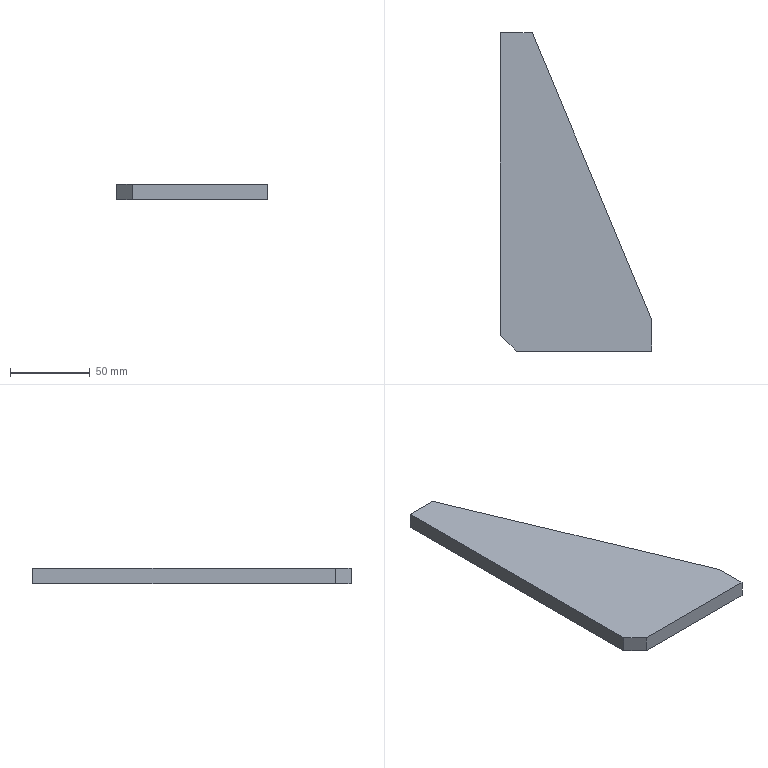Part | STEP file | 立柱底部筋Plate-200 | 1 solid | 8 faces | box 95 x 200 x 10 mm | volume 122000 mm3 | plane 8
STEP:
#1=CARTESIAN_POINT('',(0.,0.,0.));
#2=DIRECTION('',(0.,0.,1.));
#3=DIRECTION('',(1.,0.,0.));
#4=AXIS2_PLACEMENT_3D('',#1,#2,#3);
#5=CARTESIAN_POINT('',(0.,200.,-5.));
#6=VERTEX_POINT('',#5);
#7=CARTESIAN_POINT('',(0.,10.,-5.));
#8=VERTEX_POINT('',#7);
#9=CARTESIAN_POINT('',(0.,0.,-5.));
#10=DIRECTION('',(0.,-1.,0.));
#11=VECTOR('',#10,1.);
#12=LINE('',#9,#11);
#13=CARTESIAN_POINT('',(0.,0.,5.));
#14=DIRECTION('',(1.,0.,0.));
#15=DIRECTION('',(0.,0.,-1.));
#16=AXIS2_PLACEMENT_3D('',#13,#14,#15);
#17=PLANE('',#16);
#18=CARTESIAN_POINT('',(10.,0.));
#19=DIRECTION('',(0.,-1.));
#20=VECTOR('',#19,1.);
#21=LINE('',#18,#20);
#22=(GEOMETRIC_REPRESENTATION_CONTEXT(2)PARAMETRIC_REPRESENTATION_CONTEXT()REPRESENTATION_CONTEXT('',''));
#23=DEFINITIONAL_REPRESENTATION('',(#21),#22);
#24=PCURVE('',#17,#23);
#25=CARTESIAN_POINT('',(0.,0.,-5.));
#26=DIRECTION('',(0.,0.,-1.));
#27=DIRECTION('',(-1.,0.,0.));
#28=AXIS2_PLACEMENT_3D('',#25,#26,#27);
#29=PLANE('',#28);
#30=CARTESIAN_POINT('',(0.,0.));
#31=DIRECTION('',(0.,-1.));
#32=VECTOR('',#31,1.);
#33=LINE('',#30,#32);
#34=(GEOMETRIC_REPRESENTATION_CONTEXT(2)PARAMETRIC_REPRESENTATION_CONTEXT()REPRESENTATION_CONTEXT('',''));
#35=DEFINITIONAL_REPRESENTATION('',(#33),#34);
#36=PCURVE('',#29,#35);
#37=SURFACE_CURVE('',#12,(#24,#36),.PCURVE_S1.);
#38=EDGE_CURVE('',#6,#8,#37,.T.);
#39=ORIENTED_EDGE('',*,*,#38,.T.);
#40=CARTESIAN_POINT('',(0.,10.,5.));
#41=VERTEX_POINT('',#40);
#42=CARTESIAN_POINT('',(0.,10.,5.));
#43=DIRECTION('',(0.,0.,1.));
#44=VECTOR('',#43,1.);
#45=LINE('',#42,#44);
#46=CARTESIAN_POINT('',(0.,10.));
#47=DIRECTION('',(-1.,0.));
#48=VECTOR('',#47,1.);
#49=LINE('',#46,#48);
#50=(GEOMETRIC_REPRESENTATION_CONTEXT(2)PARAMETRIC_REPRESENTATION_CONTEXT()REPRESENTATION_CONTEXT('',''));
#51=DEFINITIONAL_REPRESENTATION('',(#49),#50);
#52=PCURVE('',#17,#51);
#53=CARTESIAN_POINT('',(10.,0.,5.));
#54=DIRECTION('',(0.7071,0.7071,0.));
#55=DIRECTION('',(0.,0.,-1.));
#56=AXIS2_PLACEMENT_3D('',#53,#54,#55);
#57=PLANE('',#56);
#58=CARTESIAN_POINT('',(0.,14.142));
#59=DIRECTION('',(-1.,0.));
#60=VECTOR('',#59,1.);
#61=LINE('',#58,#60);
#62=(GEOMETRIC_REPRESENTATION_CONTEXT(2)PARAMETRIC_REPRESENTATION_CONTEXT()REPRESENTATION_CONTEXT('',''));
#63=DEFINITIONAL_REPRESENTATION('',(#61),#62);
#64=PCURVE('',#57,#63);
#65=SURFACE_CURVE('',#45,(#52,#64),.PCURVE_S1.);
#66=EDGE_CURVE('',#8,#41,#65,.T.);
#67=ORIENTED_EDGE('',*,*,#66,.T.);
#68=CARTESIAN_POINT('',(0.,200.,5.));
#69=VERTEX_POINT('',#68);
#70=CARTESIAN_POINT('',(0.,0.,5.));
#71=DIRECTION('',(0.,-1.,0.));
#72=VECTOR('',#71,1.);
#73=LINE('',#70,#72);
#74=CARTESIAN_POINT('',(0.,0.));
#75=DIRECTION('',(0.,-1.));
#76=VECTOR('',#75,1.);
#77=LINE('',#74,#76);
#78=(GEOMETRIC_REPRESENTATION_CONTEXT(2)PARAMETRIC_REPRESENTATION_CONTEXT()REPRESENTATION_CONTEXT('',''));
#79=DEFINITIONAL_REPRESENTATION('',(#77),#78);
#80=PCURVE('',#17,#79);
#81=CARTESIAN_POINT('',(0.,0.,5.));
#82=DIRECTION('',(0.,0.,-1.));
#83=DIRECTION('',(-1.,0.,0.));
#84=AXIS2_PLACEMENT_3D('',#81,#82,#83);
#85=PLANE('',#84);
#86=CARTESIAN_POINT('',(0.,0.));
#87=DIRECTION('',(0.,-1.));
#88=VECTOR('',#87,1.);
#89=LINE('',#86,#88);
#90=(GEOMETRIC_REPRESENTATION_CONTEXT(2)PARAMETRIC_REPRESENTATION_CONTEXT()REPRESENTATION_CONTEXT('',''));
#91=DEFINITIONAL_REPRESENTATION('',(#89),#90);
#92=PCURVE('',#85,#91);
#93=SURFACE_CURVE('',#73,(#80,#92),.PCURVE_S1.);
#94=EDGE_CURVE('',#69,#41,#93,.T.);
#95=ORIENTED_EDGE('',*,*,#94,.F.);
#96=CARTESIAN_POINT('',(0.,200.,5.));
#97=DIRECTION('',(0.,0.,-1.));
#98=VECTOR('',#97,1.);
#99=LINE('',#96,#98);
#100=CARTESIAN_POINT('',(0.,200.));
#101=DIRECTION('',(1.,0.));
#102=VECTOR('',#101,1.);
#103=LINE('',#100,#102);
#104=(GEOMETRIC_REPRESENTATION_CONTEXT(2)PARAMETRIC_REPRESENTATION_CONTEXT()REPRESENTATION_CONTEXT('',''));
#105=DEFINITIONAL_REPRESENTATION('',(#103),#104);
#106=PCURVE('',#17,#105);
#107=CARTESIAN_POINT('',(0.,200.,5.));
#108=DIRECTION('',(0.,-1.,0.));
#109=DIRECTION('',(0.,0.,-1.));
#110=AXIS2_PLACEMENT_3D('',#107,#108,#109);
#111=PLANE('',#110);
#112=CARTESIAN_POINT('',(0.,0.));
#113=DIRECTION('',(1.,0.));
#114=VECTOR('',#113,1.);
#115=LINE('',#112,#114);
#116=(GEOMETRIC_REPRESENTATION_CONTEXT(2)PARAMETRIC_REPRESENTATION_CONTEXT()REPRESENTATION_CONTEXT('',''));
#117=DEFINITIONAL_REPRESENTATION('',(#115),#116);
#118=PCURVE('',#111,#117);
#119=SURFACE_CURVE('',#99,(#106,#118),.PCURVE_S1.);
#120=EDGE_CURVE('',#69,#6,#119,.T.);
#121=ORIENTED_EDGE('',*,*,#120,.T.);
#122=EDGE_LOOP('',(#39,#67,#95,#121));
#123=FACE_BOUND('',#122,.T.);
#124=ADVANCED_FACE('',(#123),#17,.F.);
#125=CARTESIAN_POINT('',(10.,0.,5.));
#126=VERTEX_POINT('',#125);
#127=CARTESIAN_POINT('',(95.,0.,5.));
#128=VERTEX_POINT('',#127);
#129=CARTESIAN_POINT('',(0.,0.,5.));
#130=DIRECTION('',(1.,0.,0.));
#131=VECTOR('',#130,1.);
#132=LINE('',#129,#131);
#133=CARTESIAN_POINT('',(0.,0.,5.));
#134=DIRECTION('',(0.,1.,0.));
#135=DIRECTION('',(0.,0.,1.));
#136=AXIS2_PLACEMENT_3D('',#133,#134,#135);
#137=PLANE('',#136);
#138=CARTESIAN_POINT('',(0.,0.));
#139=DIRECTION('',(0.,1.));
#140=VECTOR('',#139,1.);
#141=LINE('',#138,#140);
#142=(GEOMETRIC_REPRESENTATION_CONTEXT(2)PARAMETRIC_REPRESENTATION_CONTEXT()REPRESENTATION_CONTEXT('',''));
#143=DEFINITIONAL_REPRESENTATION('',(#141),#142);
#144=PCURVE('',#137,#143);
#145=CARTESIAN_POINT('',(0.,0.));
#146=DIRECTION('',(-1.,0.));
#147=VECTOR('',#146,1.);
#148=LINE('',#145,#147);
#149=(GEOMETRIC_REPRESENTATION_CONTEXT(2)PARAMETRIC_REPRESENTATION_CONTEXT()REPRESENTATION_CONTEXT('',''));
#150=DEFINITIONAL_REPRESENTATION('',(#148),#149);
#151=PCURVE('',#85,#150);
#152=SURFACE_CURVE('',#132,(#144,#151),.PCURVE_S1.);
#153=EDGE_CURVE('',#126,#128,#152,.T.);
#154=ORIENTED_EDGE('',*,*,#153,.F.);
#155=CARTESIAN_POINT('',(10.,0.,-5.));
#156=VERTEX_POINT('',#155);
#157=CARTESIAN_POINT('',(10.,0.,5.));
#158=DIRECTION('',(0.,0.,-1.));
#159=VECTOR('',#158,1.);
#160=LINE('',#157,#159);
#161=CARTESIAN_POINT('',(0.,10.));
#162=DIRECTION('',(-1.,0.));
#163=VECTOR('',#162,1.);
#164=LINE('',#161,#163);
#165=(GEOMETRIC_REPRESENTATION_CONTEXT(2)PARAMETRIC_REPRESENTATION_CONTEXT()REPRESENTATION_CONTEXT('',''));
#166=DEFINITIONAL_REPRESENTATION('',(#164),#165);
#167=PCURVE('',#137,#166);
#168=CARTESIAN_POINT('',(0.,0.));
#169=DIRECTION('',(1.,0.));
#170=VECTOR('',#169,1.);
#171=LINE('',#168,#170);
#172=(GEOMETRIC_REPRESENTATION_CONTEXT(2)PARAMETRIC_REPRESENTATION_CONTEXT()REPRESENTATION_CONTEXT('',''));
#173=DEFINITIONAL_REPRESENTATION('',(#171),#172);
#174=PCURVE('',#57,#173);
#175=SURFACE_CURVE('',#160,(#167,#174),.PCURVE_S1.);
#176=EDGE_CURVE('',#126,#156,#175,.T.);
#177=ORIENTED_EDGE('',*,*,#176,.T.);
#178=CARTESIAN_POINT('',(95.,0.,-5.));
#179=VERTEX_POINT('',#178);
#180=CARTESIAN_POINT('',(0.,0.,-5.));
#181=DIRECTION('',(1.,0.,0.));
#182=VECTOR('',#181,1.);
#183=LINE('',#180,#182);
#184=CARTESIAN_POINT('',(-10.,0.));
#185=DIRECTION('',(0.,1.));
#186=VECTOR('',#185,1.);
#187=LINE('',#184,#186);
#188=(GEOMETRIC_REPRESENTATION_CONTEXT(2)PARAMETRIC_REPRESENTATION_CONTEXT()REPRESENTATION_CONTEXT('',''));
#189=DEFINITIONAL_REPRESENTATION('',(#187),#188);
#190=PCURVE('',#137,#189);
#191=CARTESIAN_POINT('',(0.,0.));
#192=DIRECTION('',(-1.,0.));
#193=VECTOR('',#192,1.);
#194=LINE('',#191,#193);
#195=(GEOMETRIC_REPRESENTATION_CONTEXT(2)PARAMETRIC_REPRESENTATION_CONTEXT()REPRESENTATION_CONTEXT('',''));
#196=DEFINITIONAL_REPRESENTATION('',(#194),#195);
#197=PCURVE('',#29,#196);
#198=SURFACE_CURVE('',#183,(#190,#197),.PCURVE_S1.);
#199=EDGE_CURVE('',#156,#179,#198,.T.);
#200=ORIENTED_EDGE('',*,*,#199,.T.);
#201=CARTESIAN_POINT('',(95.,0.,5.));
#202=DIRECTION('',(0.,0.,-1.));
#203=VECTOR('',#202,1.);
#204=LINE('',#201,#203);
#205=CARTESIAN_POINT('',(0.,95.));
#206=DIRECTION('',(-1.,0.));
#207=VECTOR('',#206,1.);
#208=LINE('',#205,#207);
#209=(GEOMETRIC_REPRESENTATION_CONTEXT(2)PARAMETRIC_REPRESENTATION_CONTEXT()REPRESENTATION_CONTEXT('',''));
#210=DEFINITIONAL_REPRESENTATION('',(#208),#209);
#211=PCURVE('',#137,#210);
#212=CARTESIAN_POINT('',(95.,0.,5.));
#213=DIRECTION('',(-1.,0.,0.));
#214=DIRECTION('',(0.,-1.,0.));
#215=AXIS2_PLACEMENT_3D('',#212,#213,#214);
#216=PLANE('',#215);
#217=CARTESIAN_POINT('',(0.,0.));
#218=DIRECTION('',(0.,-1.));
#219=VECTOR('',#218,1.);
#220=LINE('',#217,#219);
#221=(GEOMETRIC_REPRESENTATION_CONTEXT(2)PARAMETRIC_REPRESENTATION_CONTEXT()REPRESENTATION_CONTEXT('',''));
#222=DEFINITIONAL_REPRESENTATION('',(#220),#221);
#223=PCURVE('',#216,#222);
#224=SURFACE_CURVE('',#204,(#211,#223),.PCURVE_S1.);
#225=EDGE_CURVE('',#128,#179,#224,.T.);
#226=ORIENTED_EDGE('',*,*,#225,.F.);
#227=EDGE_LOOP('',(#154,#177,#200,#226));
#228=FACE_BOUND('',#227,.T.);
#229=ADVANCED_FACE('',(#228),#137,.F.);
#230=CARTESIAN_POINT('',(95.,20.,-5.));
#231=VERTEX_POINT('',#230);
#232=CARTESIAN_POINT('',(95.,0.,-5.));
#233=DIRECTION('',(0.,1.,0.));
#234=VECTOR('',#233,1.);
#235=LINE('',#232,#234);
#236=CARTESIAN_POINT('',(0.,-10.));
#237=DIRECTION('',(-1.,0.));
#238=VECTOR('',#237,1.);
#239=LINE('',#236,#238);
#240=(GEOMETRIC_REPRESENTATION_CONTEXT(2)PARAMETRIC_REPRESENTATION_CONTEXT()REPRESENTATION_CONTEXT('',''));
#241=DEFINITIONAL_REPRESENTATION('',(#239),#240);
#242=PCURVE('',#216,#241);
#243=CARTESIAN_POINT('',(-95.,0.));
#244=DIRECTION('',(0.,1.));
#245=VECTOR('',#244,1.);
#246=LINE('',#243,#245);
#247=(GEOMETRIC_REPRESENTATION_CONTEXT(2)PARAMETRIC_REPRESENTATION_CONTEXT()REPRESENTATION_CONTEXT('',''));
#248=DEFINITIONAL_REPRESENTATION('',(#246),#247);
#249=PCURVE('',#29,#248);
#250=SURFACE_CURVE('',#235,(#242,#249),.PCURVE_S1.);
#251=EDGE_CURVE('',#179,#231,#250,.T.);
#252=ORIENTED_EDGE('',*,*,#251,.T.);
#253=CARTESIAN_POINT('',(95.,20.,5.));
#254=VERTEX_POINT('',#253);
#255=CARTESIAN_POINT('',(95.,20.,5.));
#256=DIRECTION('',(0.,0.,-1.));
#257=VECTOR('',#256,1.);
#258=LINE('',#255,#257);
#259=CARTESIAN_POINT('',(-20.,0.));
#260=DIRECTION('',(0.,-1.));
#261=VECTOR('',#260,1.);
#262=LINE('',#259,#261);
#263=(GEOMETRIC_REPRESENTATION_CONTEXT(2)PARAMETRIC_REPRESENTATION_CONTEXT()REPRESENTATION_CONTEXT('',''));
#264=DEFINITIONAL_REPRESENTATION('',(#262),#263);
#265=PCURVE('',#216,#264);
#266=CARTESIAN_POINT('',(95.,20.,5.));
#267=DIRECTION('',(-0.9231,-0.3846,0.));
#268=DIRECTION('',(0.3846,-0.9231,0.));
#269=AXIS2_PLACEMENT_3D('',#266,#267,#268);
#270=PLANE('',#269);
#271=CARTESIAN_POINT('',(0.,0.));
#272=DIRECTION('',(0.,-1.));
#273=VECTOR('',#272,1.);
#274=LINE('',#271,#273);
#275=(GEOMETRIC_REPRESENTATION_CONTEXT(2)PARAMETRIC_REPRESENTATION_CONTEXT()REPRESENTATION_CONTEXT('',''));
#276=DEFINITIONAL_REPRESENTATION('',(#274),#275);
#277=PCURVE('',#270,#276);
#278=SURFACE_CURVE('',#258,(#265,#277),.PCURVE_S1.);
#279=EDGE_CURVE('',#254,#231,#278,.T.);
#280=ORIENTED_EDGE('',*,*,#279,.F.);
#281=CARTESIAN_POINT('',(95.,0.,5.));
#282=DIRECTION('',(0.,1.,0.));
#283=VECTOR('',#282,1.);
#284=LINE('',#281,#283);
#285=CARTESIAN_POINT('',(0.,0.));
#286=DIRECTION('',(-1.,0.));
#287=VECTOR('',#286,1.);
#288=LINE('',#285,#287);
#289=(GEOMETRIC_REPRESENTATION_CONTEXT(2)PARAMETRIC_REPRESENTATION_CONTEXT()REPRESENTATION_CONTEXT('',''));
#290=DEFINITIONAL_REPRESENTATION('',(#288),#289);
#291=PCURVE('',#216,#290);
#292=CARTESIAN_POINT('',(-95.,0.));
#293=DIRECTION('',(0.,1.));
#294=VECTOR('',#293,1.);
#295=LINE('',#292,#294);
#296=(GEOMETRIC_REPRESENTATION_CONTEXT(2)PARAMETRIC_REPRESENTATION_CONTEXT()REPRESENTATION_CONTEXT('',''));
#297=DEFINITIONAL_REPRESENTATION('',(#295),#296);
#298=PCURVE('',#85,#297);
#299=SURFACE_CURVE('',#284,(#291,#298),.PCURVE_S1.);
#300=EDGE_CURVE('',#128,#254,#299,.T.);
#301=ORIENTED_EDGE('',*,*,#300,.F.);
#302=ORIENTED_EDGE('',*,*,#225,.T.);
#303=EDGE_LOOP('',(#252,#280,#301,#302));
#304=FACE_BOUND('',#303,.T.);
#305=ADVANCED_FACE('',(#304),#216,.F.);
#306=CARTESIAN_POINT('',(20.,200.,-5.));
#307=VERTEX_POINT('',#306);
#308=CARTESIAN_POINT('',(95.,20.,-5.));
#309=DIRECTION('',(-0.3846,0.9231,0.));
#310=VECTOR('',#309,1.);
#311=LINE('',#308,#310);
#312=CARTESIAN_POINT('',(0.,-10.));
#313=DIRECTION('',(-1.,0.));
#314=VECTOR('',#313,1.);
#315=LINE('',#312,#314);
#316=(GEOMETRIC_REPRESENTATION_CONTEXT(2)PARAMETRIC_REPRESENTATION_CONTEXT()REPRESENTATION_CONTEXT('',''));
#317=DEFINITIONAL_REPRESENTATION('',(#315),#316);
#318=PCURVE('',#270,#317);
#319=CARTESIAN_POINT('',(-95.,20.));
#320=DIRECTION('',(0.3846,0.9231));
#321=VECTOR('',#320,1.);
#322=LINE('',#319,#321);
#323=(GEOMETRIC_REPRESENTATION_CONTEXT(2)PARAMETRIC_REPRESENTATION_CONTEXT()REPRESENTATION_CONTEXT('',''));
#324=DEFINITIONAL_REPRESENTATION('',(#322),#323);
#325=PCURVE('',#29,#324);
#326=SURFACE_CURVE('',#311,(#318,#325),.PCURVE_S1.);
#327=EDGE_CURVE('',#231,#307,#326,.T.);
#328=ORIENTED_EDGE('',*,*,#327,.T.);
#329=CARTESIAN_POINT('',(20.,200.,5.));
#330=VERTEX_POINT('',#329);
#331=CARTESIAN_POINT('',(20.,200.,5.));
#332=DIRECTION('',(0.,0.,-1.));
#333=VECTOR('',#332,1.);
#334=LINE('',#331,#333);
#335=CARTESIAN_POINT('',(-195.,0.));
#336=DIRECTION('',(0.,-1.));
#337=VECTOR('',#336,1.);
#338=LINE('',#335,#337);
#339=(GEOMETRIC_REPRESENTATION_CONTEXT(2)PARAMETRIC_REPRESENTATION_CONTEXT()REPRESENTATION_CONTEXT('',''));
#340=DEFINITIONAL_REPRESENTATION('',(#338),#339);
#341=PCURVE('',#270,#340);
#342=CARTESIAN_POINT('',(0.,20.));
#343=DIRECTION('',(1.,0.));
#344=VECTOR('',#343,1.);
#345=LINE('',#342,#344);
#346=(GEOMETRIC_REPRESENTATION_CONTEXT(2)PARAMETRIC_REPRESENTATION_CONTEXT()REPRESENTATION_CONTEXT('',''));
#347=DEFINITIONAL_REPRESENTATION('',(#345),#346);
#348=PCURVE('',#111,#347);
#349=SURFACE_CURVE('',#334,(#341,#348),.PCURVE_S1.);
#350=EDGE_CURVE('',#330,#307,#349,.T.);
#351=ORIENTED_EDGE('',*,*,#350,.F.);
#352=CARTESIAN_POINT('',(95.,20.,5.));
#353=DIRECTION('',(-0.3846,0.9231,0.));
#354=VECTOR('',#353,1.);
#355=LINE('',#352,#354);
#356=CARTESIAN_POINT('',(0.,0.));
#357=DIRECTION('',(-1.,0.));
#358=VECTOR('',#357,1.);
#359=LINE('',#356,#358);
#360=(GEOMETRIC_REPRESENTATION_CONTEXT(2)PARAMETRIC_REPRESENTATION_CONTEXT()REPRESENTATION_CONTEXT('',''));
#361=DEFINITIONAL_REPRESENTATION('',(#359),#360);
#362=PCURVE('',#270,#361);
#363=CARTESIAN_POINT('',(-95.,20.));
#364=DIRECTION('',(0.3846,0.9231));
#365=VECTOR('',#364,1.);
#366=LINE('',#363,#365);
#367=(GEOMETRIC_REPRESENTATION_CONTEXT(2)PARAMETRIC_REPRESENTATION_CONTEXT()REPRESENTATION_CONTEXT('',''));
#368=DEFINITIONAL_REPRESENTATION('',(#366),#367);
#369=PCURVE('',#85,#368);
#370=SURFACE_CURVE('',#355,(#362,#369),.PCURVE_S1.);
#371=EDGE_CURVE('',#254,#330,#370,.T.);
#372=ORIENTED_EDGE('',*,*,#371,.F.);
#373=ORIENTED_EDGE('',*,*,#279,.T.);
#374=EDGE_LOOP('',(#328,#351,#372,#373));
#375=FACE_BOUND('',#374,.T.);
#376=ADVANCED_FACE('',(#375),#270,.F.);
#377=CARTESIAN_POINT('',(0.,200.,-5.));
#378=DIRECTION('',(-1.,0.,0.));
#379=VECTOR('',#378,1.);
#380=LINE('',#377,#379);
#381=CARTESIAN_POINT('',(10.,0.));
#382=DIRECTION('',(0.,-1.));
#383=VECTOR('',#382,1.);
#384=LINE('',#381,#383);
#385=(GEOMETRIC_REPRESENTATION_CONTEXT(2)PARAMETRIC_REPRESENTATION_CONTEXT()REPRESENTATION_CONTEXT('',''));
#386=DEFINITIONAL_REPRESENTATION('',(#384),#385);
#387=PCURVE('',#111,#386);
#388=CARTESIAN_POINT('',(0.,200.));
#389=DIRECTION('',(1.,0.));
#390=VECTOR('',#389,1.);
#391=LINE('',#388,#390);
#392=(GEOMETRIC_REPRESENTATION_CONTEXT(2)PARAMETRIC_REPRESENTATION_CONTEXT()REPRESENTATION_CONTEXT('',''));
#393=DEFINITIONAL_REPRESENTATION('',(#391),#392);
#394=PCURVE('',#29,#393);
#395=SURFACE_CURVE('',#380,(#387,#394),.PCURVE_S1.);
#396=EDGE_CURVE('',#307,#6,#395,.T.);
#397=ORIENTED_EDGE('',*,*,#396,.T.);
#398=ORIENTED_EDGE('',*,*,#120,.F.);
#399=CARTESIAN_POINT('',(0.,200.,5.));
#400=DIRECTION('',(-1.,0.,0.));
#401=VECTOR('',#400,1.);
#402=LINE('',#399,#401);
#403=CARTESIAN_POINT('',(0.,0.));
#404=DIRECTION('',(0.,-1.));
#405=VECTOR('',#404,1.);
#406=LINE('',#403,#405);
#407=(GEOMETRIC_REPRESENTATION_CONTEXT(2)PARAMETRIC_REPRESENTATION_CONTEXT()REPRESENTATION_CONTEXT('',''));
#408=DEFINITIONAL_REPRESENTATION('',(#406),#407);
#409=PCURVE('',#111,#408);
#410=CARTESIAN_POINT('',(0.,200.));
#411=DIRECTION('',(1.,0.));
#412=VECTOR('',#411,1.);
#413=LINE('',#410,#412);
#414=(GEOMETRIC_REPRESENTATION_CONTEXT(2)PARAMETRIC_REPRESENTATION_CONTEXT()REPRESENTATION_CONTEXT('',''));
#415=DEFINITIONAL_REPRESENTATION('',(#413),#414);
#416=PCURVE('',#85,#415);
#417=SURFACE_CURVE('',#402,(#409,#416),.PCURVE_S1.);
#418=EDGE_CURVE('',#330,#69,#417,.T.);
#419=ORIENTED_EDGE('',*,*,#418,.F.);
#420=ORIENTED_EDGE('',*,*,#350,.T.);
#421=EDGE_LOOP('',(#397,#398,#419,#420));
#422=FACE_BOUND('',#421,.T.);
#423=ADVANCED_FACE('',(#422),#111,.F.);
#424=ORIENTED_EDGE('',*,*,#94,.T.);
#425=CARTESIAN_POINT('',(10.,0.,5.));
#426=DIRECTION('',(0.7071,-0.7071,0.));
#427=VECTOR('',#426,1.);
#428=LINE('',#425,#427);
#429=CARTESIAN_POINT('',(-10.,0.));
#430=DIRECTION('',(-0.7071,-0.7071));
#431=VECTOR('',#430,1.);
#432=LINE('',#429,#431);
#433=(GEOMETRIC_REPRESENTATION_CONTEXT(2)PARAMETRIC_REPRESENTATION_CONTEXT()REPRESENTATION_CONTEXT('',''));
#434=DEFINITIONAL_REPRESENTATION('',(#432),#433);
#435=PCURVE('',#85,#434);
#436=CARTESIAN_POINT('',(0.,0.));
#437=DIRECTION('',(0.,-1.));
#438=VECTOR('',#437,1.);
#439=LINE('',#436,#438);
#440=(GEOMETRIC_REPRESENTATION_CONTEXT(2)PARAMETRIC_REPRESENTATION_CONTEXT()REPRESENTATION_CONTEXT('',''));
#441=DEFINITIONAL_REPRESENTATION('',(#439),#440);
#442=PCURVE('',#57,#441);
#443=SURFACE_CURVE('',#428,(#435,#442),.PCURVE_S1.);
#444=EDGE_CURVE('',#41,#126,#443,.T.);
#445=ORIENTED_EDGE('',*,*,#444,.T.);
#446=ORIENTED_EDGE('',*,*,#153,.T.);
#447=ORIENTED_EDGE('',*,*,#300,.T.);
#448=ORIENTED_EDGE('',*,*,#371,.T.);
#449=ORIENTED_EDGE('',*,*,#418,.T.);
#450=EDGE_LOOP('',(#424,#445,#446,#447,#448,#449));
#451=FACE_BOUND('',#450,.T.);
#452=ADVANCED_FACE('',(#451),#85,.F.);
#453=ORIENTED_EDGE('',*,*,#199,.F.);
#454=CARTESIAN_POINT('',(5.,5.,-5.));
#455=DIRECTION('',(-0.7071,0.7071,0.));
#456=VECTOR('',#455,1.);
#457=LINE('',#454,#456);
#458=CARTESIAN_POINT('',(-5.,5.));
#459=DIRECTION('',(0.7071,0.7071));
#460=VECTOR('',#459,1.);
#461=LINE('',#458,#460);
#462=(GEOMETRIC_REPRESENTATION_CONTEXT(2)PARAMETRIC_REPRESENTATION_CONTEXT()REPRESENTATION_CONTEXT('',''));
#463=DEFINITIONAL_REPRESENTATION('',(#461),#462);
#464=PCURVE('',#29,#463);
#465=CARTESIAN_POINT('',(10.,7.071));
#466=DIRECTION('',(0.,1.));
#467=VECTOR('',#466,1.);
#468=LINE('',#465,#467);
#469=(GEOMETRIC_REPRESENTATION_CONTEXT(2)PARAMETRIC_REPRESENTATION_CONTEXT()REPRESENTATION_CONTEXT('',''));
#470=DEFINITIONAL_REPRESENTATION('',(#468),#469);
#471=PCURVE('',#57,#470);
#472=SURFACE_CURVE('',#457,(#464,#471),.PCURVE_S1.);
#473=EDGE_CURVE('',#156,#8,#472,.T.);
#474=ORIENTED_EDGE('',*,*,#473,.T.);
#475=ORIENTED_EDGE('',*,*,#38,.F.);
#476=ORIENTED_EDGE('',*,*,#396,.F.);
#477=ORIENTED_EDGE('',*,*,#327,.F.);
#478=ORIENTED_EDGE('',*,*,#251,.F.);
#479=EDGE_LOOP('',(#453,#474,#475,#476,#477,#478));
#480=FACE_BOUND('',#479,.T.);
#481=ADVANCED_FACE('',(#480),#29,.T.);
#482=ORIENTED_EDGE('',*,*,#444,.F.);
#483=ORIENTED_EDGE('',*,*,#66,.F.);
#484=ORIENTED_EDGE('',*,*,#473,.F.);
#485=ORIENTED_EDGE('',*,*,#176,.F.);
#486=EDGE_LOOP('',(#482,#483,#484,#485));
#487=FACE_BOUND('',#486,.T.);
#488=ADVANCED_FACE('',(#487),#57,.F.);
#489=CLOSED_SHELL('',(#124,#229,#305,#376,#423,#452,#481,#488));
#490=MANIFOLD_SOLID_BREP('',#489);
#491=(LENGTH_UNIT()NAMED_UNIT(*)SI_UNIT(.MILLI.,.METRE.));
#492=UNCERTAINTY_MEASURE_WITH_UNIT(LENGTH_MEASURE(0.0000001),#491,'','');
#493=(NAMED_UNIT(*)PLANE_ANGLE_UNIT()SI_UNIT($,.RADIAN.));
#494=(NAMED_UNIT(*)SI_UNIT($,.STERADIAN.)SOLID_ANGLE_UNIT());
#495=(GEOMETRIC_REPRESENTATION_CONTEXT(3)GLOBAL_UNCERTAINTY_ASSIGNED_CONTEXT((#492))GLOBAL_UNIT_ASSIGNED_CONTEXT((#491,#493,#494))REPRESENTATION_CONTEXT('',''));
#496=ADVANCED_BREP_SHAPE_REPRESENTATION('',(#4,#490),#495);